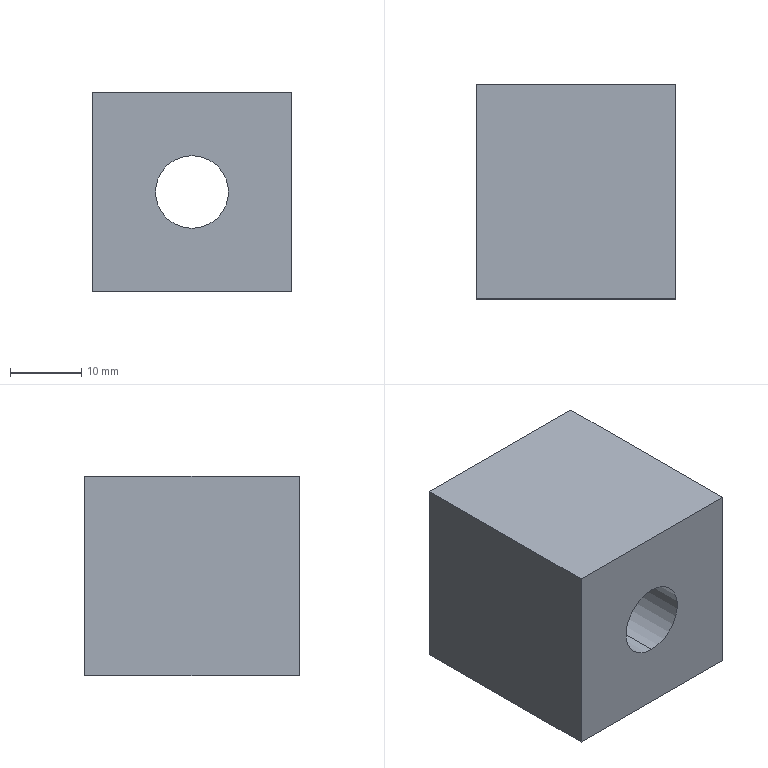Part | SolidWorks | features Extrusion 1, HoleWzd 1 | 1 solid | 8 faces | box 28 x 30 x 28 mm | volume 21069 mm3 | plane 6 | cylinder 2 | commonest cylinder face diameters 10.2 x2
STEP:
#1=CARTESIAN_POINT('',(0.,0.,-5.1));
#2=VERTEX_POINT('',#1);
#3=CARTESIAN_POINT('',(0.,0.,5.1));
#4=VERTEX_POINT('',#3);
#5=CARTESIAN_POINT('',(0.,0.,0.));
#6=DIRECTION('',(0.,1.,0.));
#7=DIRECTION('',(0.,0.,1.));
#8=AXIS2_PLACEMENT_3D('',#5,#6,#7);
#9=CIRCLE('',#8,5.1);
#10=EDGE_CURVE('',#2,#4,#9,.T.);
#11=ORIENTED_EDGE('',*,*,#10,.F.);
#12=CARTESIAN_POINT('',(0.,30.,-5.1));
#13=VERTEX_POINT('',#12);
#14=CARTESIAN_POINT('',(0.,30.,-5.1));
#15=DIRECTION('',(0.,1.,0.));
#16=VECTOR('',#15,1000.);
#17=LINE('',#14,#16);
#18=EDGE_CURVE('',#2,#13,#17,.T.);
#19=ORIENTED_EDGE('',*,*,#18,.T.);
#20=CARTESIAN_POINT('',(0.,30.,5.1));
#21=VERTEX_POINT('',#20);
#22=CARTESIAN_POINT('',(0.,30.,0.));
#23=DIRECTION('',(0.,1.,0.));
#24=DIRECTION('',(0.,0.,1.));
#25=AXIS2_PLACEMENT_3D('',#22,#23,#24);
#26=CIRCLE('',#25,5.1);
#27=EDGE_CURVE('',#13,#21,#26,.T.);
#28=ORIENTED_EDGE('',*,*,#27,.T.);
#29=CARTESIAN_POINT('',(0.,30.,5.1));
#30=DIRECTION('',(0.,1.,0.));
#31=VECTOR('',#30,1000.);
#32=LINE('',#29,#31);
#33=EDGE_CURVE('',#4,#21,#32,.T.);
#34=ORIENTED_EDGE('',*,*,#33,.F.);
#35=EDGE_LOOP('',(#11,#19,#28,#34));
#36=FACE_OUTER_BOUND('',#35,.T.);
#37=CARTESIAN_POINT('',(0.,30.,0.));
#38=DIRECTION('',(0.,1.,0.));
#39=DIRECTION('',(0.,0.,1.));
#40=AXIS2_PLACEMENT_3D('',#37,#38,#39);
#41=CYLINDRICAL_SURFACE('',#40,5.1);
#42=ADVANCED_FACE('',(#36),#41,.F.);
#43=CARTESIAN_POINT('',(0.,30.,0.));
#44=DIRECTION('',(0.,1.,0.));
#45=DIRECTION('',(0.,0.,1.));
#46=AXIS2_PLACEMENT_3D('',#43,#44,#45);
#47=CIRCLE('',#46,5.1);
#48=EDGE_CURVE('',#21,#13,#47,.T.);
#49=ORIENTED_EDGE('',*,*,#48,.F.);
#50=ORIENTED_EDGE('',*,*,#27,.F.);
#51=EDGE_LOOP('',(#49,#50));
#52=FACE_BOUND('',#51,.T.);
#53=CARTESIAN_POINT('',(14.,30.,14.));
#54=VERTEX_POINT('',#53);
#55=CARTESIAN_POINT('',(14.,30.,-14.));
#56=VERTEX_POINT('',#55);
#57=CARTESIAN_POINT('',(14.,30.,-14.));
#58=DIRECTION('',(0.,0.,-1.));
#59=VECTOR('',#58,1000.);
#60=LINE('',#57,#59);
#61=EDGE_CURVE('',#54,#56,#60,.T.);
#62=ORIENTED_EDGE('',*,*,#61,.T.);
#63=CARTESIAN_POINT('',(-14.,30.,-14.));
#64=VERTEX_POINT('',#63);
#65=CARTESIAN_POINT('',(-14.,30.,-14.));
#66=DIRECTION('',(-1.,0.,0.));
#67=VECTOR('',#66,1000.);
#68=LINE('',#65,#67);
#69=EDGE_CURVE('',#56,#64,#68,.T.);
#70=ORIENTED_EDGE('',*,*,#69,.T.);
#71=CARTESIAN_POINT('',(-14.,30.,14.));
#72=VERTEX_POINT('',#71);
#73=CARTESIAN_POINT('',(-14.,30.,-14.));
#74=DIRECTION('',(0.,0.,1.));
#75=VECTOR('',#74,1000.);
#76=LINE('',#73,#75);
#77=EDGE_CURVE('',#64,#72,#76,.T.);
#78=ORIENTED_EDGE('',*,*,#77,.T.);
#79=CARTESIAN_POINT('',(-14.,30.,14.));
#80=DIRECTION('',(1.,0.,0.));
#81=VECTOR('',#80,1000.);
#82=LINE('',#79,#81);
#83=EDGE_CURVE('',#72,#54,#82,.T.);
#84=ORIENTED_EDGE('',*,*,#83,.T.);
#85=EDGE_LOOP('',(#62,#70,#78,#84));
#86=FACE_OUTER_BOUND('',#85,.T.);
#87=CARTESIAN_POINT('',(0.,30.,0.));
#88=DIRECTION('',(0.,1.,0.));
#89=DIRECTION('',(0.,0.,1.));
#90=AXIS2_PLACEMENT_3D('',#87,#88,#89);
#91=PLANE('',#90);
#92=ADVANCED_FACE('',(#52,#86),#91,.T.);
#93=CARTESIAN_POINT('',(0.,0.,0.));
#94=DIRECTION('',(0.,1.,0.));
#95=DIRECTION('',(0.,0.,1.));
#96=AXIS2_PLACEMENT_3D('',#93,#94,#95);
#97=CIRCLE('',#96,5.1);
#98=EDGE_CURVE('',#4,#2,#97,.T.);
#99=ORIENTED_EDGE('',*,*,#98,.T.);
#100=ORIENTED_EDGE('',*,*,#10,.T.);
#101=EDGE_LOOP('',(#99,#100));
#102=FACE_BOUND('',#101,.T.);
#103=CARTESIAN_POINT('',(14.,0.,14.));
#104=VERTEX_POINT('',#103);
#105=CARTESIAN_POINT('',(14.,0.,-14.));
#106=VERTEX_POINT('',#105);
#107=CARTESIAN_POINT('',(14.,0.,-14.));
#108=DIRECTION('',(0.,0.,-1.));
#109=VECTOR('',#108,1000.);
#110=LINE('',#107,#109);
#111=EDGE_CURVE('',#104,#106,#110,.T.);
#112=ORIENTED_EDGE('',*,*,#111,.F.);
#113=CARTESIAN_POINT('',(-14.,0.,14.));
#114=VERTEX_POINT('',#113);
#115=CARTESIAN_POINT('',(-14.,0.,14.));
#116=DIRECTION('',(1.,0.,0.));
#117=VECTOR('',#116,1000.);
#118=LINE('',#115,#117);
#119=EDGE_CURVE('',#114,#104,#118,.T.);
#120=ORIENTED_EDGE('',*,*,#119,.F.);
#121=CARTESIAN_POINT('',(-14.,0.,-14.));
#122=VERTEX_POINT('',#121);
#123=CARTESIAN_POINT('',(-14.,0.,-14.));
#124=DIRECTION('',(0.,0.,1.));
#125=VECTOR('',#124,1000.);
#126=LINE('',#123,#125);
#127=EDGE_CURVE('',#122,#114,#126,.T.);
#128=ORIENTED_EDGE('',*,*,#127,.F.);
#129=CARTESIAN_POINT('',(-14.,0.,-14.));
#130=DIRECTION('',(-1.,0.,0.));
#131=VECTOR('',#130,1000.);
#132=LINE('',#129,#131);
#133=EDGE_CURVE('',#106,#122,#132,.T.);
#134=ORIENTED_EDGE('',*,*,#133,.F.);
#135=EDGE_LOOP('',(#112,#120,#128,#134));
#136=FACE_OUTER_BOUND('',#135,.T.);
#137=CARTESIAN_POINT('',(0.,0.,0.));
#138=DIRECTION('',(0.,1.,0.));
#139=DIRECTION('',(0.,0.,1.));
#140=AXIS2_PLACEMENT_3D('',#137,#138,#139);
#141=PLANE('',#140);
#142=ADVANCED_FACE('',(#102,#136),#141,.F.);
#143=ORIENTED_EDGE('',*,*,#111,.T.);
#144=CARTESIAN_POINT('',(14.,30.,-14.));
#145=DIRECTION('',(0.,-1.,0.));
#146=VECTOR('',#145,1000.);
#147=LINE('',#144,#146);
#148=EDGE_CURVE('',#56,#106,#147,.T.);
#149=ORIENTED_EDGE('',*,*,#148,.F.);
#150=ORIENTED_EDGE('',*,*,#61,.F.);
#151=CARTESIAN_POINT('',(14.,30.,14.));
#152=DIRECTION('',(0.,-1.,0.));
#153=VECTOR('',#152,1000.);
#154=LINE('',#151,#153);
#155=EDGE_CURVE('',#54,#104,#154,.T.);
#156=ORIENTED_EDGE('',*,*,#155,.T.);
#157=EDGE_LOOP('',(#143,#149,#150,#156));
#158=FACE_OUTER_BOUND('',#157,.T.);
#159=CARTESIAN_POINT('',(14.,30.,-14.));
#160=DIRECTION('',(-1.,0.,0.));
#161=DIRECTION('',(0.,0.,1.));
#162=AXIS2_PLACEMENT_3D('',#159,#160,#161);
#163=PLANE('',#162);
#164=ADVANCED_FACE('',(#158),#163,.F.);
#165=ORIENTED_EDGE('',*,*,#133,.T.);
#166=CARTESIAN_POINT('',(-14.,30.,-14.));
#167=DIRECTION('',(0.,-1.,0.));
#168=VECTOR('',#167,1000.);
#169=LINE('',#166,#168);
#170=EDGE_CURVE('',#64,#122,#169,.T.);
#171=ORIENTED_EDGE('',*,*,#170,.F.);
#172=ORIENTED_EDGE('',*,*,#69,.F.);
#173=ORIENTED_EDGE('',*,*,#148,.T.);
#174=EDGE_LOOP('',(#165,#171,#172,#173));
#175=FACE_OUTER_BOUND('',#174,.T.);
#176=CARTESIAN_POINT('',(-14.,30.,-14.));
#177=DIRECTION('',(0.,0.,1.));
#178=DIRECTION('',(1.,0.,0.));
#179=AXIS2_PLACEMENT_3D('',#176,#177,#178);
#180=PLANE('',#179);
#181=ADVANCED_FACE('',(#175),#180,.F.);
#182=ORIENTED_EDGE('',*,*,#127,.T.);
#183=CARTESIAN_POINT('',(-14.,30.,14.));
#184=DIRECTION('',(0.,-1.,0.));
#185=VECTOR('',#184,1000.);
#186=LINE('',#183,#185);
#187=EDGE_CURVE('',#72,#114,#186,.T.);
#188=ORIENTED_EDGE('',*,*,#187,.F.);
#189=ORIENTED_EDGE('',*,*,#77,.F.);
#190=ORIENTED_EDGE('',*,*,#170,.T.);
#191=EDGE_LOOP('',(#182,#188,#189,#190));
#192=FACE_OUTER_BOUND('',#191,.T.);
#193=CARTESIAN_POINT('',(-14.,30.,-14.));
#194=DIRECTION('',(1.,0.,0.));
#195=DIRECTION('',(0.,0.,-1.));
#196=AXIS2_PLACEMENT_3D('',#193,#194,#195);
#197=PLANE('',#196);
#198=ADVANCED_FACE('',(#192),#197,.F.);
#199=ORIENTED_EDGE('',*,*,#119,.T.);
#200=ORIENTED_EDGE('',*,*,#155,.F.);
#201=ORIENTED_EDGE('',*,*,#83,.F.);
#202=ORIENTED_EDGE('',*,*,#187,.T.);
#203=EDGE_LOOP('',(#199,#200,#201,#202));
#204=FACE_OUTER_BOUND('',#203,.T.);
#205=CARTESIAN_POINT('',(-14.,30.,14.));
#206=DIRECTION('',(0.,0.,-1.));
#207=DIRECTION('',(-1.,0.,0.));
#208=AXIS2_PLACEMENT_3D('',#205,#206,#207);
#209=PLANE('',#208);
#210=ADVANCED_FACE('',(#204),#209,.F.);
#211=ORIENTED_EDGE('',*,*,#18,.F.);
#212=ORIENTED_EDGE('',*,*,#98,.F.);
#213=ORIENTED_EDGE('',*,*,#33,.T.);
#214=ORIENTED_EDGE('',*,*,#48,.T.);
#215=EDGE_LOOP('',(#211,#212,#213,#214));
#216=FACE_OUTER_BOUND('',#215,.T.);
#217=CARTESIAN_POINT('',(0.,30.,0.));
#218=DIRECTION('',(0.,1.,0.));
#219=DIRECTION('',(0.,0.,1.));
#220=AXIS2_PLACEMENT_3D('',#217,#218,#219);
#221=CYLINDRICAL_SURFACE('',#220,5.1);
#222=ADVANCED_FACE('',(#216),#221,.F.);
#223=CLOSED_SHELL('',(#42,#92,#142,#164,#181,#198,#210,#222));
#224=MANIFOLD_SOLID_BREP('',#223);
#225=CARTESIAN_POINT('',(0.,0.,0.));
#226=DIRECTION('',(0.,0.,1.));
#227=DIRECTION('',(1.,0.,0.));
#228=AXIS2_PLACEMENT_3D('',#225,#226,#227);
#229=(LENGTH_UNIT()NAMED_UNIT(*)SI_UNIT(.MILLI.,.METRE.));
#230=UNCERTAINTY_MEASURE_WITH_UNIT(LENGTH_MEASURE(0.00001),#229,'','');
#231=(NAMED_UNIT(*)PLANE_ANGLE_UNIT()SI_UNIT($,.RADIAN.));
#232=(NAMED_UNIT(*)SI_UNIT($,.STERADIAN.)SOLID_ANGLE_UNIT());
#233=(GEOMETRIC_REPRESENTATION_CONTEXT(3)GLOBAL_UNCERTAINTY_ASSIGNED_CONTEXT((#230))GLOBAL_UNIT_ASSIGNED_CONTEXT((#229,#231,#232))REPRESENTATION_CONTEXT('',''));
#234=ADVANCED_BREP_SHAPE_REPRESENTATION('',(#224,#228),#233);